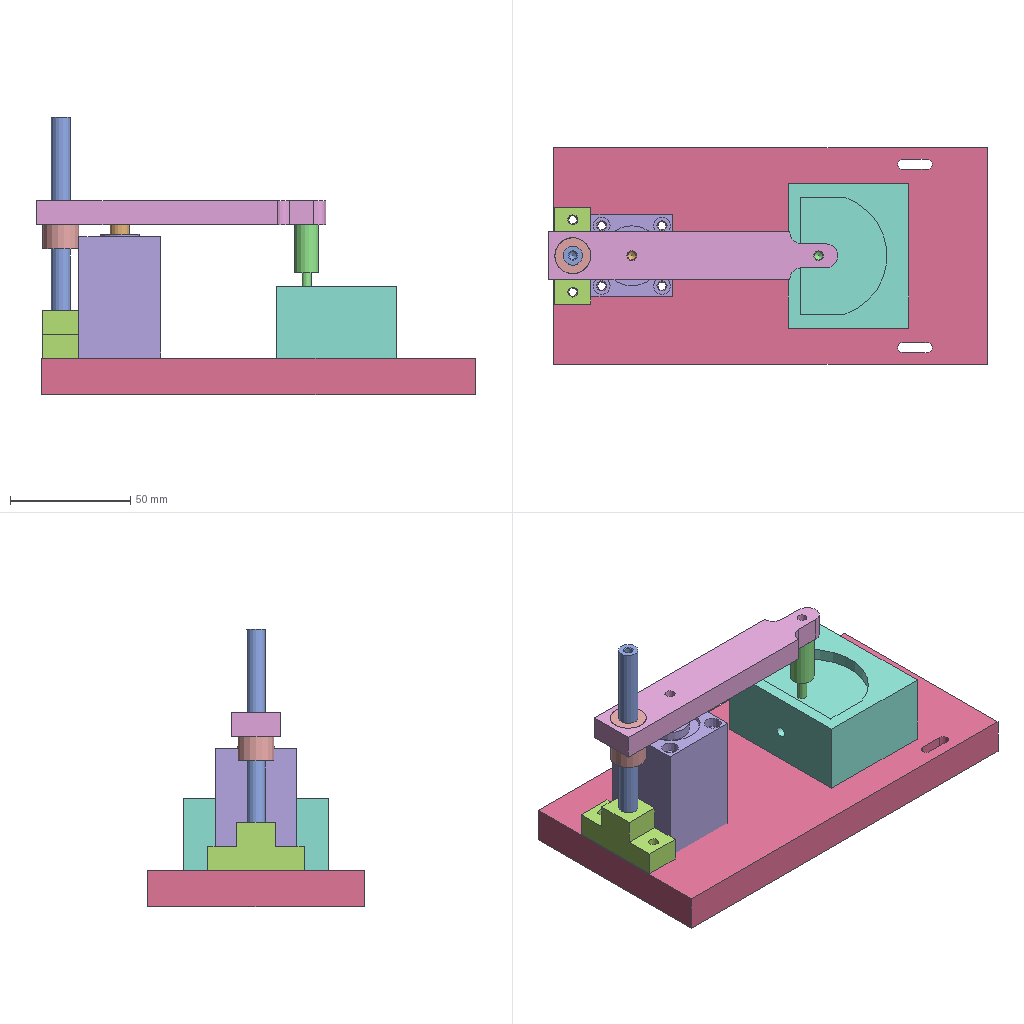Assembly | NX | 8 different items | 8 placed | box 182 x 90 x 115 mm
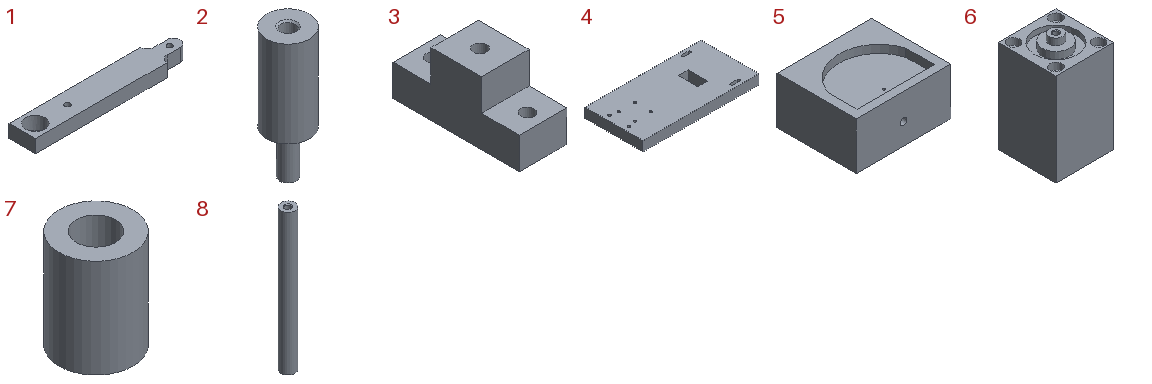Parts list (item | quantity | size | volume | features):
1 | x1 | 120 x 20 x 10 mm | 19969 mm3 | features DATUM_CSYS 5, EXTRUDE 4, SKETCH 4, BLEND 2
2 | x1 | 10 x 10 x 30 mm | 1552 mm3 | features DATUM_CSYS 3, EXTRUDE 2, SKETCH 2, HOLE PACKAGE 1, SIMPLE HOLE 1, SYMBOLIC_THREAD 1
3 | x1 | 15 x 40 x 20 mm | 7409 mm3 | features DATUM_CSYS 4, SKETCH 3, EXTRUDE 2, CBORE_HOLE 1, HOLE PACKAGE 1
4 | x1 | 180 x 90 x 15 mm | 233788 mm3 | features SIMPLE HOLE 6, SYMBOLIC_THREAD 6, DATUM_CSYS 5, SKETCH 4, EXTRUDE 3, HOLE PACKAGE 1
5 | x1 | 60 x 50 x 40 mm | 86677 mm3 | features DATUM_CSYS 6, EXTRUDE 5, SKETCH 5
6 | x1 | 34 x 34 x 59.5 mm | 58620 mm3 | features DATUM_CSYS 8, EXTRUDE 7, SKETCH 7, HOLE PACKAGE 1, Instance Feature 1, Mirror Feature 1, SIMPLE HOLE 1, SUBTRACT 1, SYMBOLIC_THREAD 1
7 | x1 | 15 x 15 x 20 mm | 2529 mm3 | features DATUM_CSYS 2, EXTRUDE 1, SKETCH 1
8 | x1 | 8 x 8 x 80 mm | 3672 mm3 | features DATUM_CSYS 2, HOLE PACKAGE 2, SIMPLE HOLE 2, SYMBOLIC_THREAD 2, EXTRUDE 1, SKETCH 1
Mates (type | each side: item.copy, entity, surface, feature):
Fix | 4.1 component
Concentric | 3.1 edge | 4.1 edge
Concentric | 8.1 edge | 3.1 edge
Concentric | 2.1 edge | 1.1 edge
Concentric | 1.1 edge | 7.1 edge
Concentric | 1.1 edge | 6.1 edge